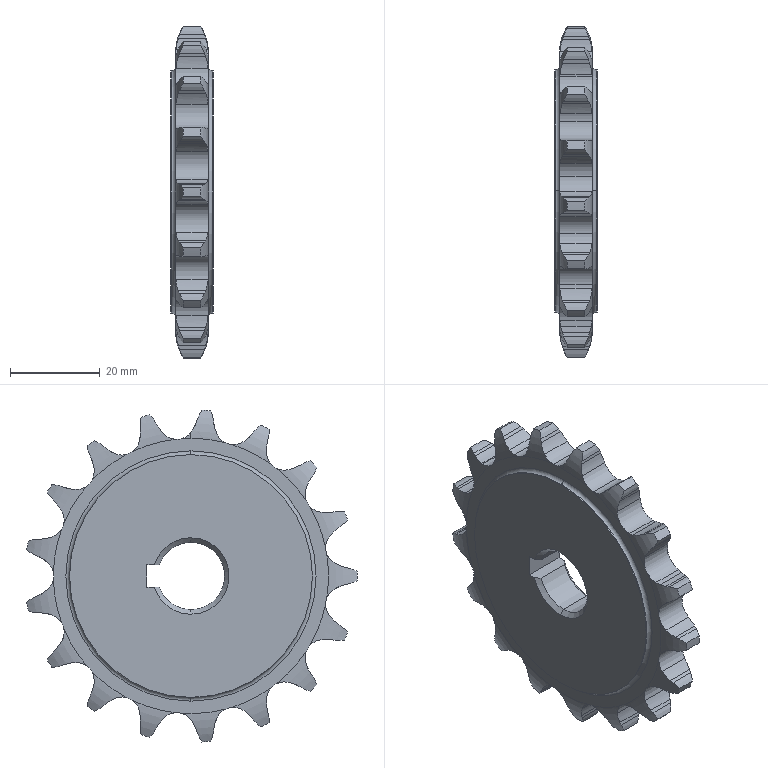Part | SolidWorks | features Chamfer 3, Cut 2, Revolution 2, CirPattern 1 | 1 solid | 203 faces | box 9.37 x 73.539 x 73.841 mm | volume 27730 mm3 | cylinder 116 | plane 41 | torus 40 | cone 6 | commonest cylinder face diameters 11.57 x35 20.732 x35 8.06 x22 74 x17 54 x4 15 x3